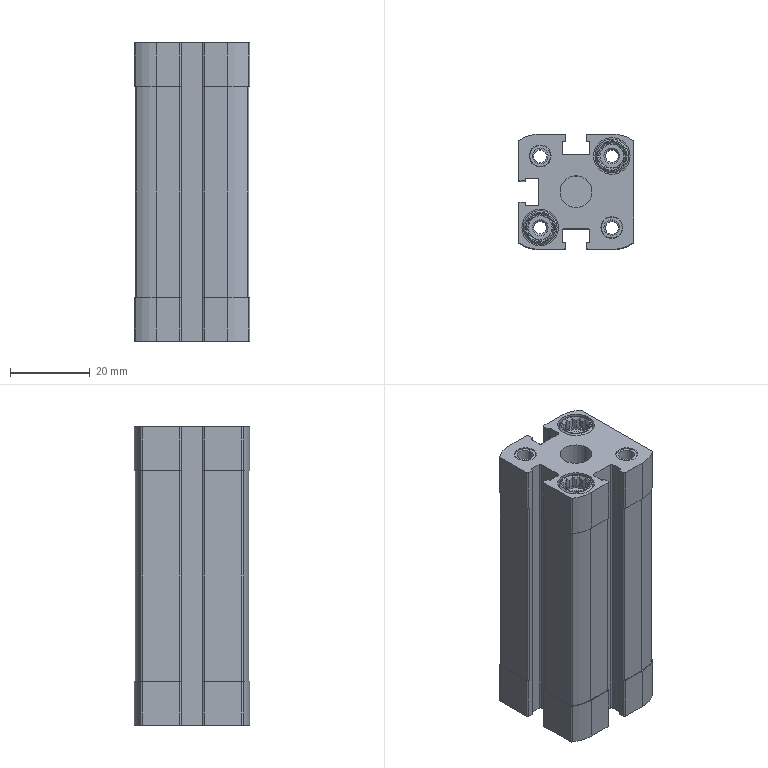Part | NX | features BREP 1 | 1 solid | 286 faces | box 29 x 29 x 75 mm | volume 39305 mm3 | plane 177 | cylinder 91 | cone 18 | commonest cylinder face diameters 0.8 x24 0.4 x12 1.2 x12 19.1 x12 3.242 x6 6 x6